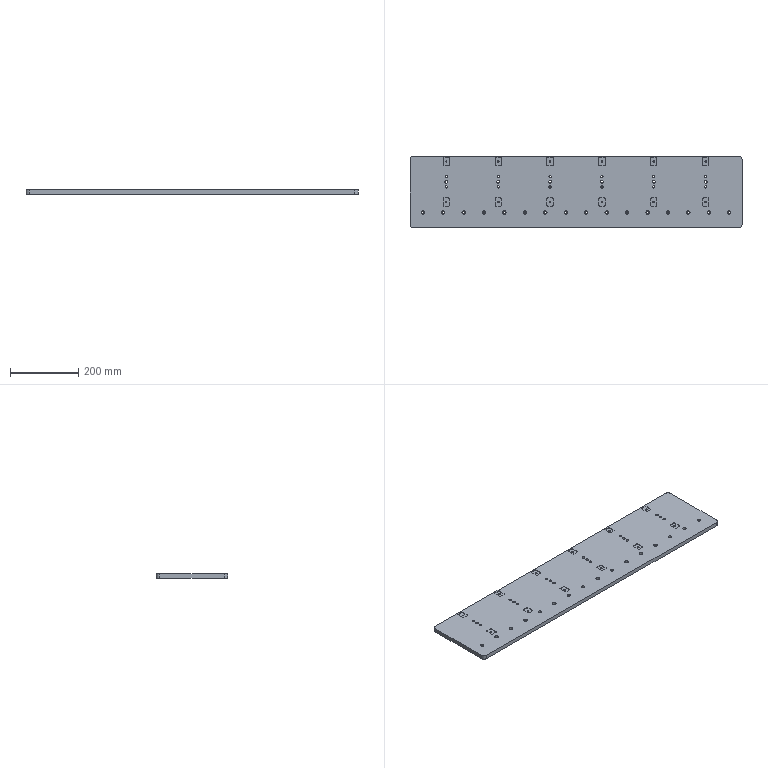Part | SolidWorks | features BaseBody 1 | 1 solid | 278 faces | box 975 x 210 x 12 mm | volume 2426074 mm3 | cylinder 176 | plane 82 | cone 20 | commonest cylinder face diameters 4 x48 5.5 x32 10 x32 3.3 x24 6.8 x24 8 x12